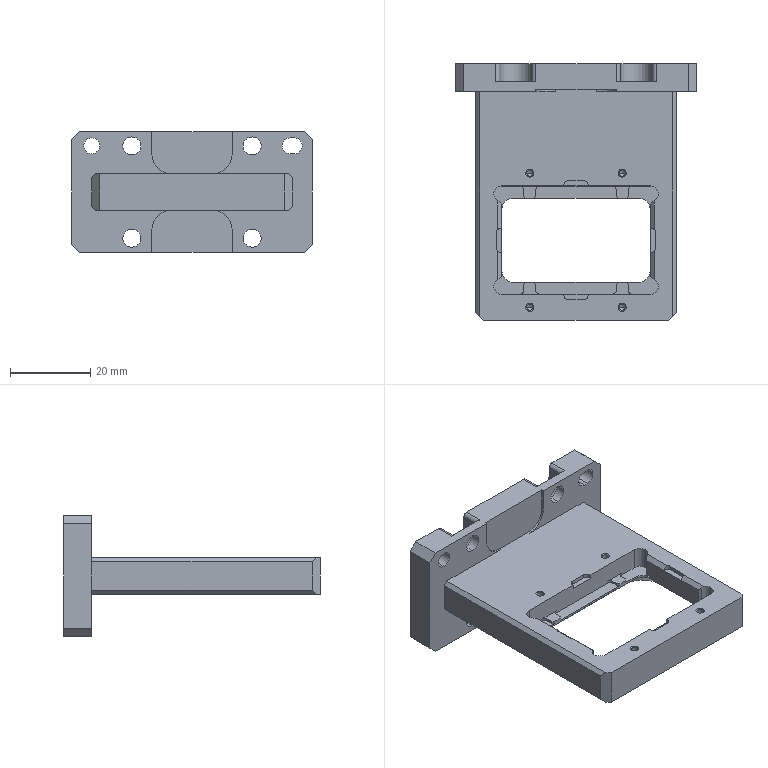NC program | NX | posted with a generic post | part box 60 x 64 x 30 mm
Lines 8343 to 9411 of 12381:
(CAVITY_MILL_COPY , TOOL : D4)
N16666 T04 M6
N16668 G54
N16670 G17 G0 G90 X4.436 Y16.5 B0. C0. S9500 M3
N16672 G43 Z30. H4
N16674 Z-9.7
N16676 G94 G1 Z-10.7 F1800.
N16678 X4.263 Y16.8
N16680 G3 X3.397 Y17.3 R1.
N16682 G1 X2.332
N16684 G2 X0.503 Y18.486 R2.012
N16686 G1 X0.5 Y18.409
N16688 Y14.403
N16690 G3 X1. Y13.537 R1.
N16692 G1 X1.3 Y13.364
N16694 Z-9.7
N16696 G0 Z30.
N16698 X4.436 Y16.3
N16700 Z-9.9
N16702 G1 Z-10.9
N16704 X4.263 Y16.6
N16706 G3 X3.397 Y17.1 R1.
N16708 G1 X2.407
N16710 G2 X0.825 Y17.87 R2.035
N16712 X0.503 Y18.486 R1.857
N16714 G1 X0.5 Y18.409
N16716 Y14.203
N16718 G3 X1. Y13.337 R1.
N16720 G1 X1.3 Y13.164
N16722 Z-9.9
N16724 G0 Z30.
N16726 X4.436 Y16.1
N16728 Z-10.1
N16730 G1 Z-11.1
N16732 X4.263 Y16.4
N16734 G3 X3.397 Y16.9 R1.
N16736 G1 X2.6
N16738 G2 X1.186 Y17.486 R2.086
N16740 G1 X0.997 Y17.674
N16742 G2 X0.553 Y18.35 R2.
N16744 G1 X0.503 Y18.485
N16746 X0.5 Y18.409
N16748 Y14.003
N16750 G3 X1. Y13.137 R1.
N16752 G1 X1.3 Y12.964
N16754 Z-10.1
N16756 G0 Z30.
N16758 X4.436 Y15.9
N16760 Z-10.3
N16762 G1 Z-11.3
N16764 X4.263 Y16.2
N16766 G3 X3.397 Y16.7 R1.
N16768 G1 X2.8
N16770 G2 X1.386 Y17.286 R2.145
N16772 G1 X0.997 Y17.674
N16774 G2 X0.531 Y18.409 R2.
N16776 G1 X0.503 Y18.485
N16778 X0.5 Y18.409
N16780 Y13.803
N16782 G3 X1. Y12.937 R1.
N16784 G1 X1.3 Y12.764
N16786 Z-10.3
N16788 G0 Z30.
N16790 X4.446 Y15.708
N16792 Z-10.5
N16794 G1 Z-11.5
N16796 X4.272 Y16.008
N16798 G3 X3.406 Y16.508 R1.
N16800 G1 X2.992
N16802 G2 X1.578 Y17.093 R2.
N16804 G1 X0.997 Y17.674
N16806 G2 X0.531 Y18.409 R2.
N16808 G1 X0.503 Y18.485
N16810 X0.5 Y18.409
N16812 Y13.61
N16814 G3 X1. Y12.744 R1.
N16816 G1 X1.3 Y12.571
N16818 Z-10.5
N16820 G0 X4.447 Y15.7 Z-10.695
N16822 G1 Z-11.695
N16824 X4.274 Y16.
N16826 G3 X3.408 Y16.5 R1.
N16828 G1 X3.
N16830 G2 X1.586 Y17.086 R2.
N16832 G1 X0.997 Y17.674
N16834 G2 X0.531 Y18.409 R2.
N16836 G1 X0.503 Y18.485
N16838 X0.5 Y18.409
N16840 Y13.603
N16842 G3 X1. Y12.737 R1.
N16844 G1 X1.3 Y12.564
N16846 Z-10.695
N16848 G0 X4.447 Y15.7 Z-10.89
N16850 G1 Z-11.89
N16852 X4.274 Y16.
N16854 G3 X3.408 Y16.5 R1.
N16856 G1 X3.
N16858 G2 X1.586 Y17.086 R2.
N16860 G1 X0.997 Y17.674
N16862 G2 X0.531 Y18.409 R2.
N16864 G1 X0.503 Y18.485
N16866 X0.5 Y18.409
N16868 Y13.603
N16870 G3 X1. Y12.737 R1.
N16872 G1 X1.3 Y12.564
N16874 Z-10.89
N16876 G0 X4.447 Y15.7 Z-11.085
N16878 G1 Z-12.085
N16880 X4.274 Y16.
N16882 G3 X3.408 Y16.5 R1.
N16884 G1 X3.
N16886 G2 X1.586 Y17.086 R2.
N16888 G1 X0.997 Y17.674
N16890 G2 X0.531 Y18.409 R2.
N16892 G1 X0.503 Y18.484
N16894 X0.5 Y18.409
N16896 Y13.603
N16898 G3 X1. Y12.737 R1.
N16900 G1 X1.3 Y12.564
N16902 Z-11.085
N16904 G0 X4.447 Y15.7 Z-11.28
N16906 G1 Z-12.28
N16908 X4.274 Y16.
N16910 G3 X3.408 Y16.5 R1.
N16912 G1 X3.
N16914 G2 X1.586 Y17.086 R2.
N16916 G1 X0.997 Y17.674
N16918 G2 X0.531 Y18.409 R2.
N16920 G1 X0.503 Y18.484
N16922 X0.5 Y18.409
N16924 Y13.603
N16926 G3 X1. Y12.737 R1.
N16928 G1 X1.3 Y12.564
N16930 Z-11.28
N16932 G0 X4.447 Y15.7 Z-11.475
N16934 G1 Z-12.475
N16936 X4.274 Y16.
N16938 G3 X3.408 Y16.5 R1.
N16940 G1 X3.
N16942 G2 X1.586 Y17.086 R2.
N16944 G1 X0.997 Y17.674
N16946 G2 X0.531 Y18.409 R2.
N16948 G1 X0.503 Y18.484
N16950 X0.5 Y18.409
N16952 Y13.603
N16954 G3 X1. Y12.737 R1.
N16956 G1 X1.3 Y12.564
N16958 Z-11.475
N16960 G0 X4.447 Y15.7 Z-11.67
N16962 G1 Z-12.67
N16964 X4.274 Y16.
N16966 G3 X3.408 Y16.5 R1.
N16968 G1 X3.
N16970 G2 X1.586 Y17.086 R2.
N16972 G1 X0.997 Y17.674
N16974 G2 X0.531 Y18.409 R2.
N16976 G1 X0.503 Y18.484
N16978 X0.5 Y18.409
N16980 Y13.603
N16982 G3 X1. Y12.737 R1.
N16984 G1 X1.3 Y12.564
N16986 Z-11.67
N16988 G0 X4.447 Y15.7 Z-11.865
N16990 G1 Z-12.865
N16992 X4.274 Y16.
N16994 G3 X3.408 Y16.5 R1.
N16996 G1 X3.
N16998 G2 X1.586 Y17.086 R2.
N17000 G1 X0.997 Y17.674
N17002 G2 X0.531 Y18.409 R2.
N17004 G1 X0.503 Y18.483
N17006 X0.5 Y18.409
N17008 Y13.603
N17010 G3 X1. Y12.737 R1.
N17012 G1 X1.3 Y12.564
N17014 Z-11.865
N17016 G0 X4.447 Y15.7 Z-12.06
N17018 G1 Z-13.06
N17020 X4.274 Y16.
N17022 G3 X3.408 Y16.5 R1.
N17024 G1 X3.
N17026 G2 X1.586 Y17.086 R2.
N17028 G1 X0.997 Y17.674
N17030 G2 X0.531 Y18.409 R2.
N17032 G1 X0.503 Y18.483
N17034 X0.5 Y18.409
N17036 Y13.603
N17038 G3 X1. Y12.737 R1.
N17040 G1 X1.3 Y12.564
N17042 Z-12.06
N17044 G0 X4.447 Y15.7 Z-12.255
N17046 G1 Z-13.255
N17048 X4.274 Y16.
N17050 G3 X3.408 Y16.5 R1.
N17052 G1 X3.
N17054 G2 X1.586 Y17.086 R2.
N17056 G1 X0.997 Y17.674
N17058 G2 X0.531 Y18.409 R2.
N17060 G1 X0.503 Y18.483
N17062 X0.5 Y18.409
N17064 Y13.603
N17066 G3 X1. Y12.737 R1.
N17068 G1 X1.3 Y12.564
N17070 Z-12.255
N17072 G0 X4.447 Y15.7 Z-12.45
N17074 G1 Z-13.45
N17076 X4.274 Y16.
N17078 G3 X3.408 Y16.5 R1.
N17080 G1 X3.
N17082 G2 X1.586 Y17.086 R2.
N17084 G1 X0.997 Y17.674
N17086 G2 X0.531 Y18.409 R2.
N17088 G1 X0.504 Y18.483
N17090 X0.5 Y18.409
N17092 Y13.603
N17094 G3 X1. Y12.737 R1.
N17096 G1 X1.3 Y12.564
N17098 Z-12.45
N17100 G0 X4.447 Y15.7 Z-12.645
N17102 G1 Z-13.645
N17104 X4.274 Y16.
N17106 G3 X3.408 Y16.5 R1.
N17108 G1 X3.
N17110 G2 X1.586 Y17.086 R2.
N17112 G1 X0.997 Y17.674
N17114 G2 X0.531 Y18.409 R2.
N17116 G1 X0.504 Y18.483
N17118 X0.5 Y18.409
N17120 Y13.603
N17122 G3 X1. Y12.737 R1.
N17124 G1 X1.3 Y12.564
N17126 Z-12.645
N17128 G0 X4.447 Y15.7 Z-12.84
N17130 G1 Z-13.84
N17132 X4.274 Y16.
N17134 G3 X3.408 Y16.5 R1.
N17136 G1 X3.
N17138 G2 X1.586 Y17.086 R2.
N17140 G1 X0.997 Y17.674
N17142 G2 X0.531 Y18.409 R2.
N17144 G1 X0.504 Y18.482
N17146 X0.5 Y18.409
N17148 Y13.603
N17150 G3 X1. Y12.737 R1.
N17152 G1 X1.3 Y12.564
N17154 Z-12.84
N17156 G0 X4.447 Y15.7 Z-13.035
N17158 G1 Z-14.035
N17160 X4.274 Y16.
N17162 G3 X3.408 Y16.5 R1.
N17164 G1 X3.
N17166 G2 X1.586 Y17.086 R2.
N17168 G1 X0.997 Y17.674
N17170 G2 X0.531 Y18.409 R2.
N17172 G1 X0.504 Y18.482
N17174 X0.5 Y18.409
N17176 Y13.603
N17178 G3 X1. Y12.737 R1.
N17180 G1 X1.3 Y12.564
N17182 Z-13.035
N17184 G0 X4.447 Y15.7 Z-13.23
N17186 G1 Z-14.23
N17188 X4.274 Y16.
N17190 G3 X3.408 Y16.5 R1.
N17192 G1 X3.
N17194 G2 X1.586 Y17.086 R2.
N17196 G1 X0.997 Y17.674
N17198 G2 X0.531 Y18.409 R2.
N17200 G1 X0.504 Y18.482
N17202 X0.5 Y18.409
N17204 Y13.603
N17206 G3 X1. Y12.737 R1.
N17208 G1 X1.3 Y12.564
N17210 Z-13.23
N17212 G0 X4.447 Y15.7 Z-13.425
N17214 G1 Z-14.425
N17216 X4.274 Y16.
N17218 G3 X3.408 Y16.5 R1.
N17220 G1 X3.
N17222 G2 X1.586 Y17.086 R2.
N17224 G1 X0.997 Y17.674
N17226 G2 X0.531 Y18.409 R2.
N17228 G1 X0.504 Y18.482
N17230 X0.5 Y18.409
N17232 Y13.603
N17234 G3 X1. Y12.737 R1.
N17236 G1 X1.3 Y12.564
N17238 Z-13.425
N17240 G0 X4.447 Y15.7 Z-13.62
N17242 G1 Z-14.62
N17244 X4.274 Y16.
N17246 G3 X3.408 Y16.5 R1.
N17248 G1 X3.
N17250 G2 X1.586 Y17.086 R2.
N17252 G1 X0.997 Y17.674
N17254 G2 X0.531 Y18.409 R2.
N17256 G1 X0.504 Y18.481
N17258 X0.5 Y18.409
N17260 Y13.603
N17262 G3 X1. Y12.737 R1.
N17264 G1 X1.3 Y12.564
N17266 Z-13.62
N17268 G0 X4.447 Y15.7 Z-13.815
N17270 G1 Z-14.815
N17272 X4.274 Y16.
N17274 G3 X3.408 Y16.5 R1.
N17276 G1 X3.
N17278 G2 X1.586 Y17.086 R2.
N17280 G1 X0.997 Y17.674
N17282 G2 X0.531 Y18.409 R2.
N17284 G1 X0.504 Y18.481
N17286 X0.5 Y18.409
N17288 Y13.603
N17290 G3 X1. Y12.737 R1.
N17292 G1 X1.3 Y12.564
N17294 Z-13.815
N17296 G0 X4.447 Y15.7 Z-14.01
N17298 G1 Z-15.01
N17300 X4.274 Y16.
N17302 G3 X3.408 Y16.5 R1.
N17304 G1 X3.
N17306 G2 X1.586 Y17.086 R2.
N17308 G1 X0.997 Y17.674
N17310 G2 X0.531 Y18.409 R2.
N17312 G1 X0.504 Y18.481
N17314 X0.5 Y18.409
N17316 Y13.603
N17318 G3 X1. Y12.737 R1.
N17320 G1 X1.3 Y12.564
N17322 Z-14.01
N17324 G0 X4.447 Y15.7 Z-14.205
N17326 G1 Z-15.205
N17328 X4.274 Y16.
N17330 G3 X3.408 Y16.5 R1.
N17332 G1 X3.
N17334 G2 X1.586 Y17.086 R2.
N17336 G1 X0.997 Y17.674
N17338 G2 X0.531 Y18.409 R2.
N17340 G1 X0.504 Y18.481
N17342 X0.5 Y18.409
N17344 Y13.603
N17346 G3 X1. Y12.737 R1.
N17348 G1 X1.3 Y12.564
N17350 Z-14.205
N17352 G0 X4.447 Y15.7 Z-14.4
N17354 G1 Z-15.4
N17356 X4.274 Y16.
N17358 G3 X3.408 Y16.5 R1.
N17360 G1 X3.
N17362 G2 X1.586 Y17.086 R2.
N17364 G1 X0.997 Y17.674
N17366 G2 X0.531 Y18.409 R2.
N17368 G1 X0.504 Y18.481
N17370 X0.5 Y18.409
N17372 Y13.603
N17374 G3 X1. Y12.737 R1.
N17376 G1 X1.3 Y12.564
N17378 Z-14.4
N17380 G0 X7.335 Y15.7 Z-14.6
N17382 G1 Z-15.6
N17384 X7.162 Y16.
N17386 G3 X6.296 Y16.5 R1.
N17388 G1 X3.
N17390 G2 X1.586 Y17.086 R2.
N17392 G1 X0.997 Y17.674
N17394 G2 X0.531 Y18.409 R2.
N17396 G1 X0.504 Y18.48
N17398 X0.5 Y18.409
N17400 Y15.
N17402 X1.
N17404 G2 X2.414 Y14.414 R2.
N17406 G1 X2.914 Y13.914
N17408 G2 X3.48 Y12.782 R2.
N17410 G3 X4.097 Y11.996 R1.
N17412 G1 X4.3 Y11.914
N17414 Z-14.6
N17416 G0 X7.335 Y15.7 Z-14.8
N17418 G1 Z-15.8
N17420 X7.162 Y16.
N17422 G3 X6.296 Y16.5 R1.
N17424 G1 X3.
N17426 G2 X1.586 Y17.086 R2.
N17428 G1 X0.997 Y17.674
N17430 G2 X0.531 Y18.409 R2.
N17432 G1 X0.504 Y18.48
N17434 X0.5 Y18.409
N17436 Y15.
N17438 X1.
N17440 G2 X2.414 Y14.414 R2.
N17442 G1 X2.914 Y13.914
N17444 G2 X3.48 Y12.782 R2.
N17446 G3 X4.097 Y11.996 R1.
N17448 G1 X4.3 Y11.914
N17450 Z-14.8
N17452 G0 X7.335 Y15.7 Z-15.
N17454 G1 Z-16.
N17456 X7.162 Y16.
N17458 G3 X6.296 Y16.5 R1.
N17460 G1 X3.
N17462 G2 X1.586 Y17.086 R2.
N17464 G1 X0.997 Y17.674
N17466 G2 X0.531 Y18.409 R2.
N17468 G1 X0.504 Y18.48
N17470 X0.5 Y18.409
N17472 Y15.
N17474 X1.
N17476 G2 X2.414 Y14.414 R2.
N17478 G1 X2.914 Y13.914
N17480 G2 X3.48 Y12.782 R2.
N17482 G3 X4.097 Y11.996 R1.
N17484 G1 X4.3 Y11.914
N17486 Z-15.
N17488 G0 X7.436 Y15.7 Z-15.194
N17490 G1 Z-16.194
N17492 X7.263 Y16.
N17494 G3 X6.397 Y16.5 R1.
N17496 G1 X4.5
N17498 G3 X3.5 Y15.5 R1.
N17500 G1 Y13.603
N17502 G3 X4. Y12.737 R1.
N17504 G1 X4.3 Y12.564
N17506 Z-15.194
N17508 G0 X7.436 Y15.7 Z-15.389
N17510 G1 Z-16.389
N17512 X7.263 Y16.
N17514 G3 X6.397 Y16.5 R1.
N17516 G1 X4.5
N17518 G3 X3.5 Y15.5 R1.
N17520 G1 Y13.603
N17522 G3 X4. Y12.737 R1.
N17524 G1 X4.3 Y12.564
N17526 Z-15.389
N17528 G0 X7.435 Y15.7 Z-15.583
N17530 G1 Z-16.583
N17532 X7.261 Y16.
N17534 G3 X6.395 Y16.5 R1.
N17536 G1 X4.5
N17538 G3 X3.5 Y15.5 R1.
N17540 G1 Y13.602
N17542 G3 X4. Y12.736 R1.
N17544 G1 X4.3 Y12.563
N17546 Z-15.583
N17548 G0 X7.435 Y15.7 Z-15.778
N17550 G1 Z-16.778
N17552 X7.261 Y16.
N17554 G3 X6.395 Y16.5 R1.
N17556 G1 X4.5
N17558 G3 X3.5 Y15.5 R1.
N17560 G1 Y13.602
N17562 G3 X4. Y12.736 R1.
N17564 G1 X4.3 Y12.563
N17566 Z-15.778
N17568 G0 X7.435 Y15.7 Z-15.972
N17570 G1 Z-16.972
N17572 X7.261 Y16.
N17574 G3 X6.395 Y16.5 R1.
N17576 G1 X4.5
N17578 G3 X3.5 Y15.5 R1.
N17580 G1 Y13.602
N17582 G3 X4. Y12.736 R1.
N17584 G1 X4.3 Y12.563
N17586 Z-15.972
N17588 G0 X7.435 Y15.7 Z-16.167
N17590 G1 Z-17.167
N17592 X7.261 Y16.
N17594 G3 X6.395 Y16.5 R1.
N17596 G1 X4.5
N17598 G3 X3.5 Y15.5 R1.
N17600 G1 Y13.602
N17602 G3 X4. Y12.736 R1.
N17604 G1 X4.3 Y12.563
N17606 Z-16.167
N17608 G0 X7.435 Y15.7 Z-16.361
N17610 G1 Z-17.361
N17612 X7.261 Y16.
N17614 G3 X6.395 Y16.5 R1.
N17616 G1 X4.5
N17618 G3 X3.5 Y15.5 R1.
N17620 G1 Y13.602
N17622 G3 X4. Y12.736 R1.
N17624 G1 X4.3 Y12.563
N17626 Z-16.361
N17628 G0 X7.435 Y15.7 Z-16.556
N17630 G1 Z-17.556
N17632 X7.261 Y16.
N17634 G3 X6.395 Y16.5 R1.
N17636 G1 X4.5
N17638 G3 X3.5 Y15.5 R1.
N17640 G1 Y13.602
N17642 G3 X4. Y12.736 R1.
N17644 G1 X4.3 Y12.563
N17646 Z-16.556
N17648 G0 X7.435 Y15.7 Z-16.75
N17650 G1 Z-17.75
N17652 X7.261 Y16.
N17654 G3 X6.395 Y16.5 R1.
N17656 G1 X4.5
N17658 G3 X3.5 Y15.5 R1.
N17660 G1 Y13.602
N17662 G3 X4. Y12.736 R1.
N17664 G1 X4.3 Y12.563
N17666 Z-16.75
N17668 G0 X7.435 Y15.7 Z-16.944
N17670 G1 Z-17.944
N17672 X7.261 Y16.
N17674 G3 X6.395 Y16.5 R1.
N17676 G1 X4.5
N17678 G3 X3.5 Y15.5 R1.
N17680 G1 Y13.602
N17682 G3 X4. Y12.736 R1.
N17684 G1 X4.3 Y12.563
N17686 Z-16.944
N17688 G0 X7.435 Y15.7 Z-17.139
N17690 G1 Z-18.139
N17692 X7.261 Y16.
N17694 G3 X6.395 Y16.5 R1.
N17696 G1 X4.5
N17698 G3 X3.5 Y15.5 R1.
N17700 G1 Y13.602
N17702 G3 X4. Y12.736 R1.
N17704 G1 X4.3 Y12.563
N17706 Z-17.139
N17708 G0 X7.435 Y15.7 Z-17.333
N17710 G1 Z-18.333
N17712 X7.261 Y16.
N17714 G3 X6.395 Y16.5 R1.
N17716 G1 X4.5
N17718 G3 X3.5 Y15.5 R1.
N17720 G1 Y13.602
N17722 G3 X4. Y12.736 R1.
N17724 G1 X4.3 Y12.563
N17726 Z-17.333
N17728 G0 X7.435 Y15.7 Z-17.528
N17730 G1 Z-18.528
N17732 X7.261 Y16.
N17734 G3 X6.395 Y16.5 R1.
N17736 G1 X4.5
N17738 G3 X3.5 Y15.5 R1.
N17740 G1 Y13.602
N17742 G3 X4. Y12.736 R1.
N17744 G1 X4.3 Y12.563
N17746 Z-17.528
N17748 G0 X7.435 Y15.7 Z-17.722
N17750 G1 Z-18.722
N17752 X7.261 Y16.
N17754 G3 X6.395 Y16.5 R1.
N17756 G1 X4.5
N17758 G3 X3.5 Y15.5 R1.
N17760 G1 Y13.602
N17762 G3 X4. Y12.736 R1.
N17764 G1 X4.3 Y12.563
N17766 Z-17.722
N17768 G0 X7.435 Y15.7 Z-17.917
N17770 G1 Z-18.917
N17772 X7.261 Y16.
N17774 G3 X6.395 Y16.5 R1.
N17776 G1 X4.5
N17778 G3 X3.5 Y15.5 R1.
N17780 G1 Y13.602
N17782 G3 X4. Y12.736 R1.
N17784 G1 X4.3 Y12.563
N17786 Z-17.917
N17788 G0 X7.435 Y15.7 Z-18.111
N17790 G1 Z-19.111
N17792 X7.261 Y16.
N17794 G3 X6.395 Y16.5 R1.
N17796 G1 X4.5
N17798 G3 X3.5 Y15.5 R1.
N17800 G1 Y13.602
N17802 G3 X4. Y12.736 R1.
N17804 G1 X4.3 Y12.563
N17806 Z-18.111
N17808 G0 X7.435 Y15.7 Z-18.306
N17810 G1 Z-19.306
N17812 X7.261 Y16.
N17814 G3 X6.395 Y16.5 R1.
N17816 G1 X4.5
N17818 G3 X3.5 Y15.5 R1.
N17820 G1 Y13.602
N17822 G3 X4. Y12.736 R1.
N17824 G1 X4.3 Y12.563
N17826 Z-18.306
N17828 G0 X7.435 Y15.7 Z-18.5
N17830 G1 Z-19.5
N17832 X7.261 Y16.
N17834 G3 X6.395 Y16.5 R1.
N17836 G1 X4.5
N17838 G3 X3.5 Y15.5 R1.
N17840 G1 Y13.602
N17842 G3 X4. Y12.736 R1.
N17844 G1 X4.3 Y12.563
N17846 Z-18.5
N17848 G0 Z30.
N17850 X12.231 Y17.
N17852 Z-9.7
N17854 G1 Z-10.7
N17856 X12.058 Y17.3
N17858 G3 X11.192 Y17.8 R1.
N17860 G1 X10.452
N17862 G2 X9.919 Y17.451 R1.856
N17864 G3 X9.322 Y16.649 R1.
N17866 G1 X9.305 Y16.502
N17868 Z-9.7
N17870 G0 Z30.
N17872 X12.54 Y17.
N17874 Z-9.9
N17876 G1 Z-10.9
N17878 X12.367 Y17.3
N17880 G3 X11.5 Y17.8 R1.
N17882 G1 X10.564
N17884 G2 X9.971 Y17.317 R1.905
N17886 G3 X9.436 Y16.472 R1.
N17888 G1 X9.429 Y16.321
N17890 Z-9.9
N17892 G0 Z30.
N17894 X12.538 Y17.
N17896 Z-10.1
N17898 G1 Z-11.1
N17900 X12.221 Y17.55
N17902 G3 X11.788 Y17.8 R0.5
N17904 G1 X10.674
N17906 G2 X10.03 Y17.176 R1.953
N17908 G3 X9.542 Y16.303 R1.
N17910 G1 X9.544 Y16.149
N17912 Z-10.1
N17914 G0 Z30.
N17916 X14.668 Y16.508
N17918 Z-9.7
N17920 G1 Z-10.7
N17922 X14.649 Y16.671
N17924 G3 X14.049 Y17.471 R1.
N17926 G2 X13.515 Y17.8 R2.13
N17928 G1 X12.806
N17930 G3 X11.94 Y17.3 R1.
N17932 G1 X11.767 Y17.
N17934 Z-9.7
N17936 G0 Z30.
N17938 X14.557 Y16.322
N17940 Z-9.9
N17942 G1 Z-10.9
N17944 X14.552 Y16.472
N17946 G3 X14.021 Y17.32 R1.
N17948 G2 X13.438 Y17.8 R1.891
N17950 G1 X12.507
N17952 G3 X11.641 Y17.3 R1.
N17954 G1 X11.467 Y17.
N17956 Z-9.9
N17958 G0 Z30.
N17960 X14.442 Y16.152
N17962 Z-10.1
N17964 G1 Z-11.1
N17966 X14.445 Y16.308
N17968 G3 X13.959 Y17.183 R1.
N17970 G2 X13.317 Y17.8 R1.986
N17972 G1 X12.213
N17974 G3 X11.347 Y17.3 R1.
N17976 G1 X11.174 Y17.
N17978 Z-10.1
N17980 G0 Z30.
N17982 X14.348 Y15.977
N17984 Z-10.3
N17986 G1 Z-11.3
N17988 X14.357 Y16.134
N17990 G3 X13.907 Y17.027 R1.
N17992 G2 X13.219 Y17.8 R1.992
N17994 G1 X10.781
N17996 G2 X10.095 Y17.027 R1.984
N17998 G3 X9.647 Y16.133 R1.
N18000 G1 X9.656 Y15.977
N18002 Z-10.3
N18004 G0 Z30.
N18006 X14.342 Y15.786
N18008 Z-10.5
N18010 G1 Z-11.5
N18012 X14.351 Y15.943
N18014 G3 X13.902 Y16.837 R1.
N18016 G2 X13.129 Y17.8 R2.003
N18018 G1 X10.871
N18020 G2 X10.079 Y16.824 R2.004
N18022 G3 X9.619 Y15.936 R1.
N18024 G1 X9.626 Y15.779
N18026 Z-10.5
N18028 G0 Z30.
N18030 X22.7 Y13.364
N18032 Z-9.7
N18034 G1 Z-10.7
N18036 X23. Y13.537
N18038 G3 X23.5 Y14.403 R1.
N18040 G1 Y18.479
N18042 G2 X21.668 Y17.3 R2.036
N18044 G1 X20.603
N18046 G3 X19.737 Y16.8 R1.
N18048 G1 X19.564 Y16.5
N18050 Z-9.7
N18052 G0 Z30.
N18054 X22.7 Y13.164
N18056 Z-9.9
N18058 G1 Z-10.9
N18060 X23. Y13.337
N18062 G3 X23.5 Y14.203 R1.
N18064 G1 Y18.477
N18066 G2 X23.175 Y17.87 R2.587
N18068 X21.593 Y17.1 R2.137
N18070 G1 X20.603
N18072 G3 X19.737 Y16.6 R1.
N18074 G1 X19.564 Y16.3
N18076 Z-9.9
N18078 G0 Z30.
N18080 X22.7 Y12.964
N18082 Z-10.1
N18084 G1 Z-11.1
N18086 X23. Y13.137
N18088 G3 X23.5 Y14.003 R1.
N18090 G1 Y18.477
N18092 X23.447 Y18.35
N18094 G2 X23.003 Y17.674 R2.
N18096 G1 X22.814 Y17.486
N18098 G2 X21.4 Y16.9 R2.
N18100 G1 X20.603
N18102 G3 X19.737 Y16.4 R1.
N18104 G1 X19.564 Y16.1
N18106 Z-10.1
N18108 G0 Z30.
N18110 X22.7 Y12.764
N18112 Z-10.3
N18114 G1 Z-11.3
N18116 X23. Y12.937
N18118 G3 X23.5 Y13.803 R1.
N18120 G1 Y18.476
N18122 X23.447 Y18.35
N18124 G2 X23.003 Y17.674 R2.
N18126 G1 X22.592 Y17.263
N18128 G2 X21.2 Y16.7 R2.192
N18130 G1 X20.603
N18132 G3 X19.737 Y16.2 R1.
N18134 G1 X19.564 Y15.9
N18136 Z-10.3
N18138 G0 Z30.
N18140 X22.7 Y12.571
N18142 Z-10.5
N18144 G1 Z-11.5
N18146 X23. Y12.744
N18148 G3 X23.5 Y13.61 R1.
N18150 G1 Y18.476
N18152 X23.447 Y18.35
N18154 G2 X23.003 Y17.674 R2.
N18156 G1 X22.422 Y17.093
N18158 G2 X21.008 Y16.508 R2.
N18160 G1 X20.594
N18162 G3 X19.728 Y16.008 R1.
N18164 G1 X19.554 Y15.708
N18166 Z-10.5
N18168 G0 X22.7 Y12.564 Z-10.695
N18170 G1 Z-11.695
N18172 X23. Y12.737
N18174 G3 X23.5 Y13.603 R1.
N18176 G1 Y18.476
N18178 X23.447 Y18.35
N18180 G2 X23.003 Y17.674 R2.
N18182 G1 X22.414 Y17.086
N18184 G2 X21. Y16.5 R2.
N18186 G1 X20.592
N18188 G3 X19.726 Y16. R1.
N18190 G1 X19.553 Y15.7
N18192 Z-10.695
N18194 G0 X22.7 Y12.564 Z-10.89
N18196 G1 Z-11.89
N18198 X23. Y12.737
N18200 G3 X23.5 Y13.603 R1.
N18202 G1 Y18.476
N18204 X23.447 Y18.35
N18206 G2 X23.003 Y17.674 R2.
N18208 G1 X22.414 Y17.086
N18210 G2 X21. Y16.5 R2.
N18212 G1 X20.592
N18214 G3 X19.726 Y16. R1.
N18216 G1 X19.553 Y15.7
N18218 Z-10.89
N18220 G0 X22.7 Y12.564 Z-11.085
N18222 G1 Z-12.085
N18224 X23. Y12.737
N18226 G3 X23.5 Y13.603 R1.
N18228 G1 Y18.476
N18230 X23.447 Y18.35
N18232 G2 X23.003 Y17.674 R2.
N18234 G1 X22.414 Y17.086
N18236 G2 X21. Y16.5 R2.
N18238 G1 X20.592
N18240 G3 X19.726 Y16. R1.
N18242 G1 X19.553 Y15.7
N18244 Z-11.085
N18246 G0 X22.7 Y12.564 Z-11.28
N18248 G1 Z-12.28
N18250 X23. Y12.737
N18252 G3 X23.5 Y13.603 R1.
N18254 G1 Y18.475
N18256 X23.447 Y18.35
N18258 G2 X23.003 Y17.674 R2.
N18260 G1 X22.414 Y17.086
N18262 G2 X21. Y16.5 R2.
N18264 G1 X20.592
N18266 G3 X19.726 Y16. R1.
N18268 G1 X19.553 Y15.7
N18270 Z-11.28
N18272 G0 X22.7 Y12.564 Z-11.475
N18274 G1 Z-12.475
N18276 X23. Y12.737
N18278 G3 X23.5 Y13.603 R1.
N18280 G1 Y18.475
N18282 X23.447 Y18.35
N18284 G2 X23.003 Y17.674 R2.
N18286 G1 X22.414 Y17.086
N18288 G2 X21. Y16.5 R2.
N18290 G1 X20.592
N18292 G3 X19.726 Y16. R1.
N18294 G1 X19.553 Y15.7
N18296 Z-11.475
N18298 G0 X22.7 Y12.564 Z-11.67
N18300 G1 Z-12.67
N18302 X23. Y12.737
N18304 G3 X23.5 Y13.603 R1.
N18306 G1 Y18.475
N18308 X23.447 Y18.35
N18310 G2 X23.003 Y17.674 R2.
N18312 G1 X22.414 Y17.086
N18314 G2 X21. Y16.5 R2.
N18316 G1 X20.592
N18318 G3 X19.726 Y16. R1.
N18320 G1 X19.553 Y15.7
N18322 Z-11.67
N18324 G0 X22.7 Y12.564 Z-11.865
N18326 G1 Z-12.865
N18328 X23. Y12.737
N18330 G3 X23.5 Y13.603 R1.
N18332 G1 Y18.475
N18334 X23.447 Y18.35
N18336 G2 X23.003 Y17.674 R2.
N18338 G1 X22.414 Y17.086
N18340 G2 X21. Y16.5 R2.
N18342 G1 X20.592
N18344 G3 X19.726 Y16. R1.
N18346 G1 X19.553 Y15.7
N18348 Z-11.865
N18350 G0 X22.7 Y12.564 Z-12.06
N18352 G1 Z-13.06
N18354 X23. Y12.737
N18356 G3 X23.5 Y13.603 R1.
N18358 G1 Y18.474
N18360 X23.447 Y18.35
N18362 G2 X23.003 Y17.674 R2.
N18364 G1 X22.414 Y17.086
N18366 G2 X21. Y16.5 R2.
N18368 G1 X20.592
N18370 G3 X19.726 Y16. R1.
N18372 G1 X19.553 Y15.7
N18374 Z-12.06
N18376 G0 X22.7 Y12.564 Z-12.255
N18378 G1 Z-13.255
N18380 X23. Y12.737
N18382 G3 X23.5 Y13.603 R1.
N18384 G1 Y18.474
N18386 X23.447 Y18.35
N18388 G2 X23.003 Y17.674 R2.
N18390 G1 X22.414 Y17.086
N18392 G2 X21. Y16.5 R2.
N18394 G1 X20.592
N18396 G3 X19.726 Y16. R1.
N18398 G1 X19.553 Y15.7
N18400 Z-12.255
N18402 G0 X22.7 Y12.564 Z-12.45
N18404 G1 Z-13.45
N18406 X23. Y12.737
N18408 G3 X23.5 Y13.603 R1.
N18410 G1 Y18.474
N18412 X23.447 Y18.35
N18414 G2 X23.003 Y17.674 R2.
N18416 G1 X22.414 Y17.086
N18418 G2 X21. Y16.5 R2.
N18420 G1 X20.592
N18422 G3 X19.726 Y16. R1.
N18424 G1 X19.553 Y15.7
N18426 Z-12.45
N18428 G0 X22.7 Y12.564 Z-12.645
N18430 G1 Z-13.645
N18432 X23. Y12.737
N18434 G3 X23.5 Y13.603 R1.
N18436 G1 Y18.474
N18438 X23.447 Y18.35
N18440 G2 X23.003 Y17.674 R2.
N18442 G1 X22.414 Y17.086
N18444 G2 X21. Y16.5 R2.
N18446 G1 X20.592
N18448 G3 X19.726 Y16. R1.
N18450 G1 X19.553 Y15.7
N18452 Z-12.645
N18454 G0 X22.7 Y12.564 Z-12.84
N18456 G1 Z-13.84
N18458 X23. Y12.737
N18460 G3 X23.5 Y13.603 R1.
N18462 G1 Y18.474
N18464 X23.447 Y18.35
N18466 G2 X23.003 Y17.674 R2.
N18468 G1 X22.414 Y17.086
N18470 G2 X21. Y16.5 R2.
N18472 G1 X20.592
N18474 G3 X19.726 Y16. R1.
N18476 G1 X19.553 Y15.7
N18478 Z-12.84
N18480 G0 X22.7 Y12.564 Z-13.035
N18482 G1 Z-14.035
N18484 X23. Y12.737
N18486 G3 X23.5 Y13.603 R1.
N18488 G1 Y18.473
N18490 X23.447 Y18.35
N18492 G2 X23.003 Y17.674 R2.
N18494 G1 X22.414 Y17.086
N18496 G2 X21. Y16.5 R2.
N18498 G1 X20.592
N18500 G3 X19.726 Y16. R1.
N18502 G1 X19.553 Y15.7
N18504 Z-13.035
N18506 G0 X22.7 Y12.564 Z-13.23
N18508 G1 Z-14.23
N18510 X23. Y12.737
N18512 G3 X23.5 Y13.603 R1.
N18514 G1 Y18.473
N18516 X23.448 Y18.352
N18518 G2 X23.003 Y17.674 R2.
N18520 G1 X22.414 Y17.086
N18522 G2 X21. Y16.5 R2.
N18524 G1 X20.592
N18526 G3 X19.726 Y16. R1.
N18528 G1 X19.553 Y15.7
N18530 Z-13.23
N18532 G0 X22.7 Y12.564 Z-13.425
N18534 G1 Z-14.425
N18536 X23. Y12.737
N18538 G3 X23.5 Y13.603 R1.
N18540 G1 Y18.473
N18542 X23.469 Y18.409
N18544 G2 X23.003 Y17.674 R2.
N18546 G1 X22.414 Y17.086
N18548 G2 X21. Y16.5 R2.
N18550 G1 X20.592
N18552 G3 X19.726 Y16. R1.
N18554 G1 X19.553 Y15.7
N18556 Z-13.425
N18558 G0 X22.7 Y12.564 Z-13.62
N18560 G1 Z-14.62
N18562 X23. Y12.737
N18564 G3 X23.5 Y13.603 R1.
N18566 G1 Y18.473
N18568 X23.469 Y18.409
N18570 G2 X23.003 Y17.674 R2.
N18572 G1 X22.414 Y17.086
N18574 G2 X21. Y16.5 R2.
N18576 G1 X20.592
N18578 G3 X19.726 Y16. R1.
N18580 G1 X19.553 Y15.7
N18582 Z-13.62
N18584 G0 X22.7 Y12.564 Z-13.815
N18586 G1 Z-14.815
N18588 X23. Y12.737
N18590 G3 X23.5 Y13.603 R1.
N18592 G1 Y18.472
N18594 X23.469 Y18.409
N18596 G2 X23.003 Y17.674 R2.
N18598 G1 X22.414 Y17.086
N18600 G2 X21. Y16.5 R2.
N18602 G1 X20.592
N18604 G3 X19.726 Y16. R1.
N18606 G1 X19.553 Y15.7
N18608 Z-13.815
N18610 G0 X22.7 Y12.564 Z-14.01
N18612 G1 Z-15.01
N18614 X23. Y12.737
N18616 G3 X23.5 Y13.603 R1.
N18618 G1 Y18.472
N18620 X23.469 Y18.409
N18622 G2 X23.003 Y17.674 R2.
N18624 G1 X22.414 Y17.086
N18626 G2 X21. Y16.5 R2.
N18628 G1 X20.592
N18630 G3 X19.726 Y16. R1.
N18632 G1 X19.553 Y15.7
N18634 Z-14.01
N18636 G0 X22.7 Y12.564 Z-14.205
N18638 G1 Z-15.205
N18640 X23. Y12.737
N18642 G3 X23.5 Y13.603 R1.
N18644 G1 Y18.472
N18646 X23.469 Y18.409
N18648 G2 X23.003 Y17.674 R2.
N18650 G1 X22.414 Y17.086
N18652 G2 X21. Y16.5 R2.
N18654 G1 X20.592
N18656 G3 X19.726 Y16. R1.
N18658 G1 X19.553 Y15.7
N18660 Z-14.205
N18662 G0 X22.7 Y12.564 Z-14.4
N18664 G1 Z-15.4
N18666 X23. Y12.737
N18668 G3 X23.5 Y13.603 R1.
N18670 G1 Y18.472
N18672 X23.469 Y18.409
N18674 G2 X23.003 Y17.674 R2.
N18676 G1 X22.414 Y17.086
N18678 G2 X21. Y16.5 R2.
N18680 G1 X20.592
N18682 G3 X19.726 Y16. R1.
N18684 G1 X19.553 Y15.7
N18686 Z-14.4
N18688 G0 X19.7 Y11.914 Z-14.6
N18690 G1 Z-15.6
N18692 X19.903 Y11.996
N18694 G3 X20.52 Y12.782 R1.
N18696 G2 X21.086 Y13.914 R2.
N18698 G1 X21.586 Y14.414
N18700 G2 X23. Y15. R2.
N18702 G1 X23.5
N18704 Y18.472
N18706 X23.464 Y18.394
N18708 G2 X23.003 Y17.674 R2.
N18710 G1 X22.414 Y17.086
N18712 G2 X21. Y16.5 R2.
N18714 G1 X17.704
N18716 G3 X16.838 Y16. R1.
N18718 G1 X16.665 Y15.7
N18720 Z-14.6
N18722 G0 X19.7 Y11.914 Z-14.8
N18724 G1 Z-15.8
N18726 X19.903 Y11.996
N18728 G3 X20.52 Y12.782 R1.
N18730 G2 X21.086 Y13.914 R2.
N18732 G1 X21.586 Y14.414
N18734 G2 X23. Y15. R2.
N18736 G1 X23.5
N18738 Y18.471
N18740 X23.466 Y18.4
N18742 G2 X23.003 Y17.674 R2.
N18744 G1 X22.414 Y17.086
N18746 G2 X21. Y16.5 R2.
N18748 G1 X17.704
N18750 G3 X16.838 Y16. R1.
N18752 G1 X16.665 Y15.7
N18754 Z-14.8
N18756 G0 X19.7 Y11.914 Z-15.
N18758 G1 Z-16.
N18760 X19.903 Y11.996
N18762 G3 X20.52 Y12.782 R1.
N18764 G2 X21.086 Y13.914 R2.
N18766 G1 X21.586 Y14.414
N18768 G2 X23. Y15. R2.
N18770 G1 X23.5
N18772 Y18.471
N18774 X23.466 Y18.4
N18776 G2 X23.003 Y17.674 R2.
N18778 G1 X22.414 Y17.086
N18780 G2 X21. Y16.5 R2.
N18782 G1 X17.704
N18784 G3 X16.838 Y16. R1.
N18786 G1 X16.665 Y15.7
N18788 Z-15.
N18790 G0 X19.7 Y12.564 Z-15.194
N18792 G1 Z-16.194
N18794 X20. Y12.737
N18796 G3 X20.5 Y13.603 R1.